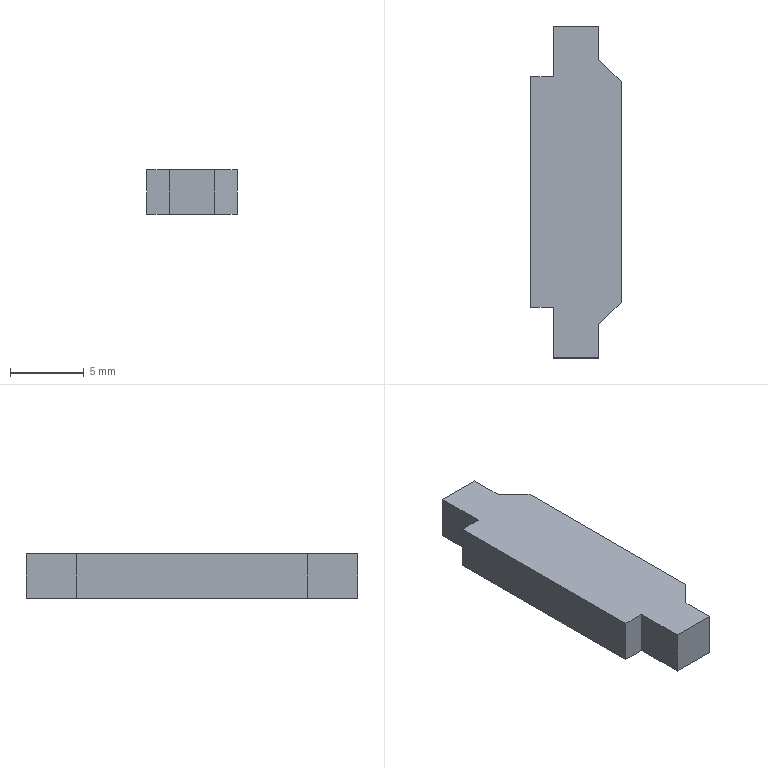Part | SolidWorks | features BaseBody 1 | 1 solid | 14 faces | box 6.137 x 22.551 x 3 mm | volume 356.006 mm3 | plane 14
STEP:
#1=CARTESIAN_POINT('',(-41.419,-12.813,-1.5));
#2=VERTEX_POINT('',#1);
#3=CARTESIAN_POINT('',(-42.956,-11.276,-1.5));
#4=VERTEX_POINT('',#3);
#5=CARTESIAN_POINT('',(-42.956,-11.276,-1.5));
#6=DIRECTION('',(-0.7071,0.7071,0.));
#7=VECTOR('',#6,1000.);
#8=LINE('',#5,#7);
#9=EDGE_CURVE('',#2,#4,#8,.T.);
#10=ORIENTED_EDGE('',*,*,#9,.F.);
#11=CARTESIAN_POINT('',(-41.419,-27.793,-1.5));
#12=VERTEX_POINT('',#11);
#13=CARTESIAN_POINT('',(-41.419,-12.813,-1.5));
#14=DIRECTION('',(0.,1.,0.));
#15=VECTOR('',#14,1000.);
#16=LINE('',#13,#15);
#17=EDGE_CURVE('',#12,#2,#16,.T.);
#18=ORIENTED_EDGE('',*,*,#17,.F.);
#19=CARTESIAN_POINT('',(-42.956,-29.329,-1.5));
#20=VERTEX_POINT('',#19);
#21=CARTESIAN_POINT('',(-41.419,-27.793,-1.5));
#22=DIRECTION('',(0.7071,0.7071,0.));
#23=VECTOR('',#22,1000.);
#24=LINE('',#21,#23);
#25=EDGE_CURVE('',#20,#12,#24,.T.);
#26=ORIENTED_EDGE('',*,*,#25,.F.);
#27=CARTESIAN_POINT('',(-42.956,-31.578,-1.5));
#28=VERTEX_POINT('',#27);
#29=CARTESIAN_POINT('',(-42.956,-29.329,-1.5));
#30=DIRECTION('',(0.,1.,0.));
#31=VECTOR('',#30,1000.);
#32=LINE('',#29,#31);
#33=EDGE_CURVE('',#28,#20,#32,.T.);
#34=ORIENTED_EDGE('',*,*,#33,.F.);
#35=CARTESIAN_POINT('',(-46.035,-31.578,-1.5));
#36=VERTEX_POINT('',#35);
#37=CARTESIAN_POINT('',(-42.956,-31.578,-1.5));
#38=DIRECTION('',(1.,0.,0.));
#39=VECTOR('',#38,1000.);
#40=LINE('',#37,#39);
#41=EDGE_CURVE('',#36,#28,#40,.T.);
#42=ORIENTED_EDGE('',*,*,#41,.F.);
#43=CARTESIAN_POINT('',(-46.035,-28.143,-1.5));
#44=VERTEX_POINT('',#43);
#45=CARTESIAN_POINT('',(-46.035,-31.578,-1.5));
#46=DIRECTION('',(0.,-1.,0.));
#47=VECTOR('',#46,1000.);
#48=LINE('',#45,#47);
#49=EDGE_CURVE('',#44,#36,#48,.T.);
#50=ORIENTED_EDGE('',*,*,#49,.F.);
#51=CARTESIAN_POINT('',(-47.556,-28.143,-1.5));
#52=VERTEX_POINT('',#51);
#53=CARTESIAN_POINT('',(-46.035,-28.143,-1.5));
#54=DIRECTION('',(1.,0.,0.));
#55=VECTOR('',#54,1000.);
#56=LINE('',#53,#55);
#57=EDGE_CURVE('',#52,#44,#56,.T.);
#58=ORIENTED_EDGE('',*,*,#57,.F.);
#59=CARTESIAN_POINT('',(-47.556,-12.463,-1.5));
#60=VERTEX_POINT('',#59);
#61=CARTESIAN_POINT('',(-47.556,-28.143,-1.5));
#62=DIRECTION('',(0.,-1.,0.));
#63=VECTOR('',#62,1000.);
#64=LINE('',#61,#63);
#65=EDGE_CURVE('',#60,#52,#64,.T.);
#66=ORIENTED_EDGE('',*,*,#65,.F.);
#67=CARTESIAN_POINT('',(-46.035,-12.463,-1.5));
#68=VERTEX_POINT('',#67);
#69=CARTESIAN_POINT('',(-47.556,-12.463,-1.5));
#70=DIRECTION('',(-1.,0.,0.));
#71=VECTOR('',#70,1000.);
#72=LINE('',#69,#71);
#73=EDGE_CURVE('',#68,#60,#72,.T.);
#74=ORIENTED_EDGE('',*,*,#73,.F.);
#75=CARTESIAN_POINT('',(-46.035,-9.027,-1.5));
#76=VERTEX_POINT('',#75);
#77=CARTESIAN_POINT('',(-46.035,-12.463,-1.5));
#78=DIRECTION('',(0.,-1.,0.));
#79=VECTOR('',#78,1000.);
#80=LINE('',#77,#79);
#81=EDGE_CURVE('',#76,#68,#80,.T.);
#82=ORIENTED_EDGE('',*,*,#81,.F.);
#83=CARTESIAN_POINT('',(-42.956,-9.027,-1.5));
#84=VERTEX_POINT('',#83);
#85=CARTESIAN_POINT('',(-46.035,-9.027,-1.5));
#86=DIRECTION('',(-1.,0.,0.));
#87=VECTOR('',#86,1000.);
#88=LINE('',#85,#87);
#89=EDGE_CURVE('',#84,#76,#88,.T.);
#90=ORIENTED_EDGE('',*,*,#89,.F.);
#91=CARTESIAN_POINT('',(-42.956,-9.027,-1.5));
#92=DIRECTION('',(0.,1.,0.));
#93=VECTOR('',#92,1000.);
#94=LINE('',#91,#93);
#95=EDGE_CURVE('',#4,#84,#94,.T.);
#96=ORIENTED_EDGE('',*,*,#95,.F.);
#97=EDGE_LOOP('',(#10,#18,#26,#34,#42,#50,#58,#66,#74,#82,#90,#96));
#98=FACE_OUTER_BOUND('',#97,.T.);
#99=CARTESIAN_POINT('',(0.,0.,-1.5));
#100=DIRECTION('',(0.,0.,-1.));
#101=DIRECTION('',(0.,-1.,0.));
#102=AXIS2_PLACEMENT_3D('',#99,#100,#101);
#103=PLANE('',#102);
#104=ADVANCED_FACE('',(#98),#103,.T.);
#105=CARTESIAN_POINT('',(-41.419,-12.813,1.5));
#106=VERTEX_POINT('',#105);
#107=CARTESIAN_POINT('',(-42.956,-11.276,1.5));
#108=VERTEX_POINT('',#107);
#109=CARTESIAN_POINT('',(-42.956,-11.276,1.5));
#110=DIRECTION('',(-0.7071,0.7071,0.));
#111=VECTOR('',#110,1000.);
#112=LINE('',#109,#111);
#113=EDGE_CURVE('',#106,#108,#112,.T.);
#114=ORIENTED_EDGE('',*,*,#113,.T.);
#115=CARTESIAN_POINT('',(-42.956,-9.027,1.5));
#116=VERTEX_POINT('',#115);
#117=CARTESIAN_POINT('',(-42.956,-9.027,1.5));
#118=DIRECTION('',(0.,1.,0.));
#119=VECTOR('',#118,1000.);
#120=LINE('',#117,#119);
#121=EDGE_CURVE('',#108,#116,#120,.T.);
#122=ORIENTED_EDGE('',*,*,#121,.T.);
#123=CARTESIAN_POINT('',(-46.035,-9.027,1.5));
#124=VERTEX_POINT('',#123);
#125=CARTESIAN_POINT('',(-46.035,-9.027,1.5));
#126=DIRECTION('',(-1.,0.,0.));
#127=VECTOR('',#126,1000.);
#128=LINE('',#125,#127);
#129=EDGE_CURVE('',#116,#124,#128,.T.);
#130=ORIENTED_EDGE('',*,*,#129,.T.);
#131=CARTESIAN_POINT('',(-46.035,-12.463,1.5));
#132=VERTEX_POINT('',#131);
#133=CARTESIAN_POINT('',(-46.035,-12.463,1.5));
#134=DIRECTION('',(0.,-1.,0.));
#135=VECTOR('',#134,1000.);
#136=LINE('',#133,#135);
#137=EDGE_CURVE('',#124,#132,#136,.T.);
#138=ORIENTED_EDGE('',*,*,#137,.T.);
#139=CARTESIAN_POINT('',(-47.556,-12.463,1.5));
#140=VERTEX_POINT('',#139);
#141=CARTESIAN_POINT('',(-47.556,-12.463,1.5));
#142=DIRECTION('',(-1.,0.,0.));
#143=VECTOR('',#142,1000.);
#144=LINE('',#141,#143);
#145=EDGE_CURVE('',#132,#140,#144,.T.);
#146=ORIENTED_EDGE('',*,*,#145,.T.);
#147=CARTESIAN_POINT('',(-47.556,-28.143,1.5));
#148=VERTEX_POINT('',#147);
#149=CARTESIAN_POINT('',(-47.556,-28.143,1.5));
#150=DIRECTION('',(0.,-1.,0.));
#151=VECTOR('',#150,1000.);
#152=LINE('',#149,#151);
#153=EDGE_CURVE('',#140,#148,#152,.T.);
#154=ORIENTED_EDGE('',*,*,#153,.T.);
#155=CARTESIAN_POINT('',(-46.035,-28.143,1.5));
#156=VERTEX_POINT('',#155);
#157=CARTESIAN_POINT('',(-46.035,-28.143,1.5));
#158=DIRECTION('',(1.,0.,0.));
#159=VECTOR('',#158,1000.);
#160=LINE('',#157,#159);
#161=EDGE_CURVE('',#148,#156,#160,.T.);
#162=ORIENTED_EDGE('',*,*,#161,.T.);
#163=CARTESIAN_POINT('',(-46.035,-31.578,1.5));
#164=VERTEX_POINT('',#163);
#165=CARTESIAN_POINT('',(-46.035,-31.578,1.5));
#166=DIRECTION('',(0.,-1.,0.));
#167=VECTOR('',#166,1000.);
#168=LINE('',#165,#167);
#169=EDGE_CURVE('',#156,#164,#168,.T.);
#170=ORIENTED_EDGE('',*,*,#169,.T.);
#171=CARTESIAN_POINT('',(-42.956,-31.578,1.5));
#172=VERTEX_POINT('',#171);
#173=CARTESIAN_POINT('',(-42.956,-31.578,1.5));
#174=DIRECTION('',(1.,0.,0.));
#175=VECTOR('',#174,1000.);
#176=LINE('',#173,#175);
#177=EDGE_CURVE('',#164,#172,#176,.T.);
#178=ORIENTED_EDGE('',*,*,#177,.T.);
#179=CARTESIAN_POINT('',(-42.956,-29.329,1.5));
#180=VERTEX_POINT('',#179);
#181=CARTESIAN_POINT('',(-42.956,-29.329,1.5));
#182=DIRECTION('',(0.,1.,0.));
#183=VECTOR('',#182,1000.);
#184=LINE('',#181,#183);
#185=EDGE_CURVE('',#172,#180,#184,.T.);
#186=ORIENTED_EDGE('',*,*,#185,.T.);
#187=CARTESIAN_POINT('',(-41.419,-27.793,1.5));
#188=VERTEX_POINT('',#187);
#189=CARTESIAN_POINT('',(-41.419,-27.793,1.5));
#190=DIRECTION('',(0.7071,0.7071,0.));
#191=VECTOR('',#190,1000.);
#192=LINE('',#189,#191);
#193=EDGE_CURVE('',#180,#188,#192,.T.);
#194=ORIENTED_EDGE('',*,*,#193,.T.);
#195=CARTESIAN_POINT('',(-41.419,-12.813,1.5));
#196=DIRECTION('',(0.,1.,0.));
#197=VECTOR('',#196,1000.);
#198=LINE('',#195,#197);
#199=EDGE_CURVE('',#188,#106,#198,.T.);
#200=ORIENTED_EDGE('',*,*,#199,.T.);
#201=EDGE_LOOP('',(#114,#122,#130,#138,#146,#154,#162,#170,#178,#186,#194,#200));
#202=FACE_OUTER_BOUND('',#201,.T.);
#203=CARTESIAN_POINT('',(0.,0.,1.5));
#204=DIRECTION('',(0.,0.,-1.));
#205=DIRECTION('',(0.,-1.,0.));
#206=AXIS2_PLACEMENT_3D('',#203,#204,#205);
#207=PLANE('',#206);
#208=ADVANCED_FACE('',(#202),#207,.F.);
#209=ORIENTED_EDGE('',*,*,#17,.T.);
#210=CARTESIAN_POINT('',(-41.419,-12.813,1.5));
#211=DIRECTION('',(0.,0.,-1.));
#212=VECTOR('',#211,1000.);
#213=LINE('',#210,#212);
#214=EDGE_CURVE('',#106,#2,#213,.T.);
#215=ORIENTED_EDGE('',*,*,#214,.F.);
#216=ORIENTED_EDGE('',*,*,#199,.F.);
#217=CARTESIAN_POINT('',(-41.419,-27.793,1.5));
#218=DIRECTION('',(0.,0.,-1.));
#219=VECTOR('',#218,1000.);
#220=LINE('',#217,#219);
#221=EDGE_CURVE('',#188,#12,#220,.T.);
#222=ORIENTED_EDGE('',*,*,#221,.T.);
#223=EDGE_LOOP('',(#209,#215,#216,#222));
#224=FACE_OUTER_BOUND('',#223,.T.);
#225=CARTESIAN_POINT('',(-41.419,-12.813,1.5));
#226=DIRECTION('',(-1.,0.,0.));
#227=DIRECTION('',(0.,0.,1.));
#228=AXIS2_PLACEMENT_3D('',#225,#226,#227);
#229=PLANE('',#228);
#230=ADVANCED_FACE('',(#224),#229,.F.);
#231=ORIENTED_EDGE('',*,*,#25,.T.);
#232=ORIENTED_EDGE('',*,*,#221,.F.);
#233=ORIENTED_EDGE('',*,*,#193,.F.);
#234=CARTESIAN_POINT('',(-42.956,-29.329,1.5));
#235=DIRECTION('',(0.,0.,-1.));
#236=VECTOR('',#235,1000.);
#237=LINE('',#234,#236);
#238=EDGE_CURVE('',#180,#20,#237,.T.);
#239=ORIENTED_EDGE('',*,*,#238,.T.);
#240=EDGE_LOOP('',(#231,#232,#233,#239));
#241=FACE_OUTER_BOUND('',#240,.T.);
#242=CARTESIAN_POINT('',(-41.419,-27.793,1.5));
#243=DIRECTION('',(-0.7071,0.7071,0.));
#244=DIRECTION('',(0.,0.,1.));
#245=AXIS2_PLACEMENT_3D('',#242,#243,#244);
#246=PLANE('',#245);
#247=ADVANCED_FACE('',(#241),#246,.F.);
#248=ORIENTED_EDGE('',*,*,#33,.T.);
#249=ORIENTED_EDGE('',*,*,#238,.F.);
#250=ORIENTED_EDGE('',*,*,#185,.F.);
#251=CARTESIAN_POINT('',(-42.956,-31.578,1.5));
#252=DIRECTION('',(0.,0.,-1.));
#253=VECTOR('',#252,1000.);
#254=LINE('',#251,#253);
#255=EDGE_CURVE('',#172,#28,#254,.T.);
#256=ORIENTED_EDGE('',*,*,#255,.T.);
#257=EDGE_LOOP('',(#248,#249,#250,#256));
#258=FACE_OUTER_BOUND('',#257,.T.);
#259=CARTESIAN_POINT('',(-42.956,-29.329,1.5));
#260=DIRECTION('',(-1.,0.,0.));
#261=DIRECTION('',(0.,0.,1.));
#262=AXIS2_PLACEMENT_3D('',#259,#260,#261);
#263=PLANE('',#262);
#264=ADVANCED_FACE('',(#258),#263,.F.);
#265=ORIENTED_EDGE('',*,*,#41,.T.);
#266=ORIENTED_EDGE('',*,*,#255,.F.);
#267=ORIENTED_EDGE('',*,*,#177,.F.);
#268=CARTESIAN_POINT('',(-46.035,-31.578,1.5));
#269=DIRECTION('',(0.,0.,-1.));
#270=VECTOR('',#269,1000.);
#271=LINE('',#268,#270);
#272=EDGE_CURVE('',#164,#36,#271,.T.);
#273=ORIENTED_EDGE('',*,*,#272,.T.);
#274=EDGE_LOOP('',(#265,#266,#267,#273));
#275=FACE_OUTER_BOUND('',#274,.T.);
#276=CARTESIAN_POINT('',(-42.956,-31.578,1.5));
#277=DIRECTION('',(0.,1.,0.));
#278=DIRECTION('',(1.,0.,0.));
#279=AXIS2_PLACEMENT_3D('',#276,#277,#278);
#280=PLANE('',#279);
#281=ADVANCED_FACE('',(#275),#280,.F.);
#282=ORIENTED_EDGE('',*,*,#49,.T.);
#283=ORIENTED_EDGE('',*,*,#272,.F.);
#284=ORIENTED_EDGE('',*,*,#169,.F.);
#285=CARTESIAN_POINT('',(-46.035,-28.143,1.5));
#286=DIRECTION('',(0.,0.,-1.));
#287=VECTOR('',#286,1000.);
#288=LINE('',#285,#287);
#289=EDGE_CURVE('',#156,#44,#288,.T.);
#290=ORIENTED_EDGE('',*,*,#289,.T.);
#291=EDGE_LOOP('',(#282,#283,#284,#290));
#292=FACE_OUTER_BOUND('',#291,.T.);
#293=CARTESIAN_POINT('',(-46.035,-31.578,1.5));
#294=DIRECTION('',(1.,0.,0.));
#295=DIRECTION('',(0.,1.,0.));
#296=AXIS2_PLACEMENT_3D('',#293,#294,#295);
#297=PLANE('',#296);
#298=ADVANCED_FACE('',(#292),#297,.F.);
#299=ORIENTED_EDGE('',*,*,#57,.T.);
#300=ORIENTED_EDGE('',*,*,#289,.F.);
#301=ORIENTED_EDGE('',*,*,#161,.F.);
#302=CARTESIAN_POINT('',(-47.556,-28.143,1.5));
#303=DIRECTION('',(0.,0.,-1.));
#304=VECTOR('',#303,1000.);
#305=LINE('',#302,#304);
#306=EDGE_CURVE('',#148,#52,#305,.T.);
#307=ORIENTED_EDGE('',*,*,#306,.T.);
#308=EDGE_LOOP('',(#299,#300,#301,#307));
#309=FACE_OUTER_BOUND('',#308,.T.);
#310=CARTESIAN_POINT('',(-46.035,-28.143,1.5));
#311=DIRECTION('',(0.,1.,0.));
#312=DIRECTION('',(1.,0.,0.));
#313=AXIS2_PLACEMENT_3D('',#310,#311,#312);
#314=PLANE('',#313);
#315=ADVANCED_FACE('',(#309),#314,.F.);
#316=ORIENTED_EDGE('',*,*,#65,.T.);
#317=ORIENTED_EDGE('',*,*,#306,.F.);
#318=ORIENTED_EDGE('',*,*,#153,.F.);
#319=CARTESIAN_POINT('',(-47.556,-12.463,1.5));
#320=DIRECTION('',(0.,0.,-1.));
#321=VECTOR('',#320,1000.);
#322=LINE('',#319,#321);
#323=EDGE_CURVE('',#140,#60,#322,.T.);
#324=ORIENTED_EDGE('',*,*,#323,.T.);
#325=EDGE_LOOP('',(#316,#317,#318,#324));
#326=FACE_OUTER_BOUND('',#325,.T.);
#327=CARTESIAN_POINT('',(-47.556,-28.143,1.5));
#328=DIRECTION('',(1.,0.,0.));
#329=DIRECTION('',(0.,1.,0.));
#330=AXIS2_PLACEMENT_3D('',#327,#328,#329);
#331=PLANE('',#330);
#332=ADVANCED_FACE('',(#326),#331,.F.);
#333=ORIENTED_EDGE('',*,*,#73,.T.);
#334=ORIENTED_EDGE('',*,*,#323,.F.);
#335=ORIENTED_EDGE('',*,*,#145,.F.);
#336=CARTESIAN_POINT('',(-46.035,-12.463,1.5));
#337=DIRECTION('',(0.,0.,-1.));
#338=VECTOR('',#337,1000.);
#339=LINE('',#336,#338);
#340=EDGE_CURVE('',#132,#68,#339,.T.);
#341=ORIENTED_EDGE('',*,*,#340,.T.);
#342=EDGE_LOOP('',(#333,#334,#335,#341));
#343=FACE_OUTER_BOUND('',#342,.T.);
#344=CARTESIAN_POINT('',(-47.556,-12.463,1.5));
#345=DIRECTION('',(0.,-1.,0.));
#346=DIRECTION('',(0.,0.,-1.));
#347=AXIS2_PLACEMENT_3D('',#344,#345,#346);
#348=PLANE('',#347);
#349=ADVANCED_FACE('',(#343),#348,.F.);
#350=ORIENTED_EDGE('',*,*,#81,.T.);
#351=ORIENTED_EDGE('',*,*,#340,.F.);
#352=ORIENTED_EDGE('',*,*,#137,.F.);
#353=CARTESIAN_POINT('',(-46.035,-9.027,1.5));
#354=DIRECTION('',(0.,0.,-1.));
#355=VECTOR('',#354,1000.);
#356=LINE('',#353,#355);
#357=EDGE_CURVE('',#124,#76,#356,.T.);
#358=ORIENTED_EDGE('',*,*,#357,.T.);
#359=EDGE_LOOP('',(#350,#351,#352,#358));
#360=FACE_OUTER_BOUND('',#359,.T.);
#361=CARTESIAN_POINT('',(-46.035,-12.463,1.5));
#362=DIRECTION('',(1.,0.,0.));
#363=DIRECTION('',(0.,1.,0.));
#364=AXIS2_PLACEMENT_3D('',#361,#362,#363);
#365=PLANE('',#364);
#366=ADVANCED_FACE('',(#360),#365,.F.);
#367=ORIENTED_EDGE('',*,*,#89,.T.);
#368=ORIENTED_EDGE('',*,*,#357,.F.);
#369=ORIENTED_EDGE('',*,*,#129,.F.);
#370=CARTESIAN_POINT('',(-42.956,-9.027,1.5));
#371=DIRECTION('',(0.,0.,-1.));
#372=VECTOR('',#371,1000.);
#373=LINE('',#370,#372);
#374=EDGE_CURVE('',#116,#84,#373,.T.);
#375=ORIENTED_EDGE('',*,*,#374,.T.);
#376=EDGE_LOOP('',(#367,#368,#369,#375));
#377=FACE_OUTER_BOUND('',#376,.T.);
#378=CARTESIAN_POINT('',(-46.035,-9.027,1.5));
#379=DIRECTION('',(0.,-1.,0.));
#380=DIRECTION('',(0.,0.,-1.));
#381=AXIS2_PLACEMENT_3D('',#378,#379,#380);
#382=PLANE('',#381);
#383=ADVANCED_FACE('',(#377),#382,.F.);
#384=ORIENTED_EDGE('',*,*,#95,.T.);
#385=ORIENTED_EDGE('',*,*,#374,.F.);
#386=ORIENTED_EDGE('',*,*,#121,.F.);
#387=CARTESIAN_POINT('',(-42.956,-11.276,1.5));
#388=DIRECTION('',(0.,0.,-1.));
#389=VECTOR('',#388,1000.);
#390=LINE('',#387,#389);
#391=EDGE_CURVE('',#108,#4,#390,.T.);
#392=ORIENTED_EDGE('',*,*,#391,.T.);
#393=EDGE_LOOP('',(#384,#385,#386,#392));
#394=FACE_OUTER_BOUND('',#393,.T.);
#395=CARTESIAN_POINT('',(-42.956,-9.027,1.5));
#396=DIRECTION('',(-1.,0.,0.));
#397=DIRECTION('',(0.,0.,1.));
#398=AXIS2_PLACEMENT_3D('',#395,#396,#397);
#399=PLANE('',#398);
#400=ADVANCED_FACE('',(#394),#399,.F.);
#401=ORIENTED_EDGE('',*,*,#9,.T.);
#402=ORIENTED_EDGE('',*,*,#391,.F.);
#403=ORIENTED_EDGE('',*,*,#113,.F.);
#404=ORIENTED_EDGE('',*,*,#214,.T.);
#405=EDGE_LOOP('',(#401,#402,#403,#404));
#406=FACE_OUTER_BOUND('',#405,.T.);
#407=CARTESIAN_POINT('',(-42.956,-11.276,1.5));
#408=DIRECTION('',(-0.7071,-0.7071,0.));
#409=DIRECTION('',(-0.7071,0.7071,0.));
#410=AXIS2_PLACEMENT_3D('',#407,#408,#409);
#411=PLANE('',#410);
#412=ADVANCED_FACE('',(#406),#411,.F.);
#413=CLOSED_SHELL('',(#104,#208,#230,#247,#264,#281,#298,#315,#332,#349,#366,#383,#400,#412));
#414=MANIFOLD_SOLID_BREP('',#413);
#415=CARTESIAN_POINT('',(0.,0.,0.));
#416=DIRECTION('',(0.,0.,1.));
#417=DIRECTION('',(1.,0.,0.));
#418=AXIS2_PLACEMENT_3D('',#415,#416,#417);
#419=(LENGTH_UNIT()NAMED_UNIT(*)SI_UNIT(.MILLI.,.METRE.));
#420=UNCERTAINTY_MEASURE_WITH_UNIT(LENGTH_MEASURE(0.00001),#419,'','');
#421=(NAMED_UNIT(*)PLANE_ANGLE_UNIT()SI_UNIT($,.RADIAN.));
#422=(NAMED_UNIT(*)SI_UNIT($,.STERADIAN.)SOLID_ANGLE_UNIT());
#423=(GEOMETRIC_REPRESENTATION_CONTEXT(3)GLOBAL_UNCERTAINTY_ASSIGNED_CONTEXT((#420))GLOBAL_UNIT_ASSIGNED_CONTEXT((#419,#421,#422))REPRESENTATION_CONTEXT('',''));
#424=ADVANCED_BREP_SHAPE_REPRESENTATION('',(#414,#418),#423);